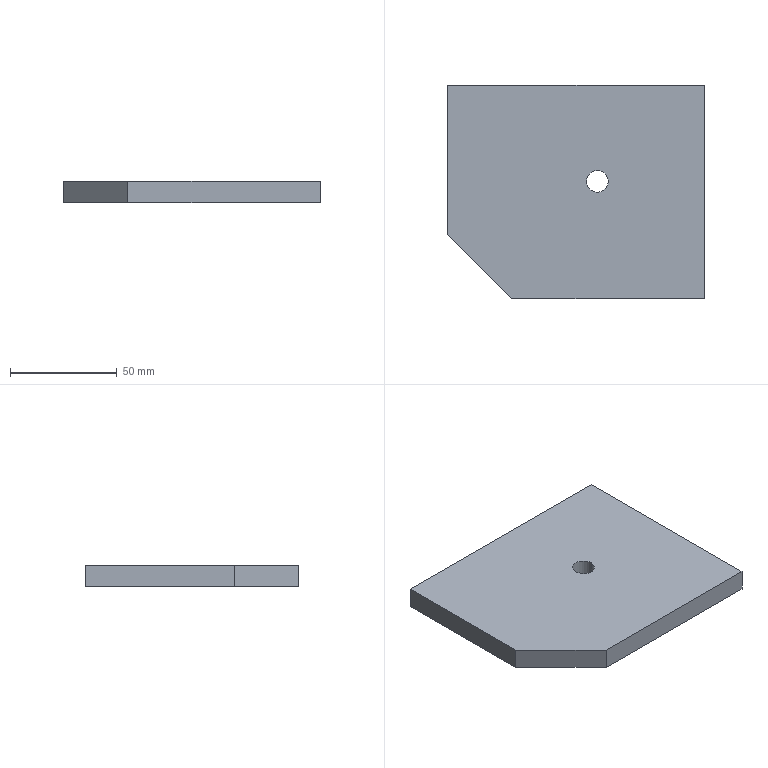Part | SolidWorks | features Extrusion 1, HoleWzd 1 | 1 solid | 9 faces | box 120 x 100 x 10 mm | volume 114683 mm3 | plane 7 | cylinder 2 | commonest cylinder face diameters 10.2 x2
STEP:
#1=CARTESIAN_POINT('',(4.055,5.704,0.));
#2=VERTEX_POINT('',#1);
#3=CARTESIAN_POINT('',(14.255,5.704,0.));
#4=VERTEX_POINT('',#3);
#5=CARTESIAN_POINT('',(9.155,5.704,0.));
#6=DIRECTION('',(0.,0.,1.));
#7=DIRECTION('',(1.,0.,0.));
#8=AXIS2_PLACEMENT_3D('',#5,#6,#7);
#9=CIRCLE('',#8,5.1);
#10=EDGE_CURVE('',#2,#4,#9,.T.);
#11=ORIENTED_EDGE('',*,*,#10,.F.);
#12=CARTESIAN_POINT('',(4.055,5.704,10.));
#13=VERTEX_POINT('',#12);
#14=CARTESIAN_POINT('',(4.055,5.704,10.));
#15=DIRECTION('',(0.,0.,1.));
#16=VECTOR('',#15,1000.);
#17=LINE('',#14,#16);
#18=EDGE_CURVE('',#2,#13,#17,.T.);
#19=ORIENTED_EDGE('',*,*,#18,.T.);
#20=CARTESIAN_POINT('',(14.255,5.704,10.));
#21=VERTEX_POINT('',#20);
#22=CARTESIAN_POINT('',(9.155,5.704,10.));
#23=DIRECTION('',(0.,0.,1.));
#24=DIRECTION('',(1.,0.,0.));
#25=AXIS2_PLACEMENT_3D('',#22,#23,#24);
#26=CIRCLE('',#25,5.1);
#27=EDGE_CURVE('',#13,#21,#26,.T.);
#28=ORIENTED_EDGE('',*,*,#27,.T.);
#29=CARTESIAN_POINT('',(14.255,5.704,10.));
#30=DIRECTION('',(0.,0.,1.));
#31=VECTOR('',#30,1000.);
#32=LINE('',#29,#31);
#33=EDGE_CURVE('',#4,#21,#32,.T.);
#34=ORIENTED_EDGE('',*,*,#33,.F.);
#35=EDGE_LOOP('',(#11,#19,#28,#34));
#36=FACE_OUTER_BOUND('',#35,.T.);
#37=CARTESIAN_POINT('',(9.155,5.704,10.));
#38=DIRECTION('',(0.,0.,1.));
#39=DIRECTION('',(1.,0.,0.));
#40=AXIS2_PLACEMENT_3D('',#37,#38,#39);
#41=CYLINDRICAL_SURFACE('',#40,5.1);
#42=ADVANCED_FACE('',(#36),#41,.F.);
#43=CARTESIAN_POINT('',(59.155,-49.296,0.));
#44=VERTEX_POINT('',#43);
#45=CARTESIAN_POINT('',(59.155,50.704,0.));
#46=VERTEX_POINT('',#45);
#47=CARTESIAN_POINT('',(59.155,50.704,0.));
#48=DIRECTION('',(0.,1.,0.));
#49=VECTOR('',#48,1000.);
#50=LINE('',#47,#49);
#51=EDGE_CURVE('',#44,#46,#50,.T.);
#52=ORIENTED_EDGE('',*,*,#51,.T.);
#53=CARTESIAN_POINT('',(59.155,50.704,10.));
#54=VERTEX_POINT('',#53);
#55=CARTESIAN_POINT('',(59.155,50.704,10.));
#56=DIRECTION('',(0.,0.,-1.));
#57=VECTOR('',#56,1000.);
#58=LINE('',#55,#57);
#59=EDGE_CURVE('',#54,#46,#58,.T.);
#60=ORIENTED_EDGE('',*,*,#59,.F.);
#61=CARTESIAN_POINT('',(59.155,-49.296,10.));
#62=VERTEX_POINT('',#61);
#63=CARTESIAN_POINT('',(59.155,50.704,10.));
#64=DIRECTION('',(0.,1.,0.));
#65=VECTOR('',#64,1000.);
#66=LINE('',#63,#65);
#67=EDGE_CURVE('',#62,#54,#66,.T.);
#68=ORIENTED_EDGE('',*,*,#67,.F.);
#69=CARTESIAN_POINT('',(59.155,-49.296,10.));
#70=DIRECTION('',(0.,0.,-1.));
#71=VECTOR('',#70,1000.);
#72=LINE('',#69,#71);
#73=EDGE_CURVE('',#62,#44,#72,.T.);
#74=ORIENTED_EDGE('',*,*,#73,.T.);
#75=EDGE_LOOP('',(#52,#60,#68,#74));
#76=FACE_OUTER_BOUND('',#75,.T.);
#77=CARTESIAN_POINT('',(59.155,50.704,10.));
#78=DIRECTION('',(-1.,0.,0.));
#79=DIRECTION('',(0.,-1.,0.));
#80=AXIS2_PLACEMENT_3D('',#77,#78,#79);
#81=PLANE('',#80);
#82=ADVANCED_FACE('',(#76),#81,.F.);
#83=CARTESIAN_POINT('',(-60.845,50.704,0.));
#84=VERTEX_POINT('',#83);
#85=CARTESIAN_POINT('',(-60.845,50.704,0.));
#86=DIRECTION('',(-1.,0.,0.));
#87=VECTOR('',#86,1000.);
#88=LINE('',#85,#87);
#89=EDGE_CURVE('',#46,#84,#88,.T.);
#90=ORIENTED_EDGE('',*,*,#89,.T.);
#91=CARTESIAN_POINT('',(-60.845,50.704,10.));
#92=VERTEX_POINT('',#91);
#93=CARTESIAN_POINT('',(-60.845,50.704,10.));
#94=DIRECTION('',(0.,0.,-1.));
#95=VECTOR('',#94,1000.);
#96=LINE('',#93,#95);
#97=EDGE_CURVE('',#92,#84,#96,.T.);
#98=ORIENTED_EDGE('',*,*,#97,.F.);
#99=CARTESIAN_POINT('',(-60.845,50.704,10.));
#100=DIRECTION('',(-1.,0.,0.));
#101=VECTOR('',#100,1000.);
#102=LINE('',#99,#101);
#103=EDGE_CURVE('',#54,#92,#102,.T.);
#104=ORIENTED_EDGE('',*,*,#103,.F.);
#105=ORIENTED_EDGE('',*,*,#59,.T.);
#106=EDGE_LOOP('',(#90,#98,#104,#105));
#107=FACE_OUTER_BOUND('',#106,.T.);
#108=CARTESIAN_POINT('',(-60.845,50.704,10.));
#109=DIRECTION('',(0.,-1.,0.));
#110=DIRECTION('',(0.,0.,-1.));
#111=AXIS2_PLACEMENT_3D('',#108,#109,#110);
#112=PLANE('',#111);
#113=ADVANCED_FACE('',(#107),#112,.F.);
#114=CARTESIAN_POINT('',(-60.845,-19.296,0.));
#115=VERTEX_POINT('',#114);
#116=CARTESIAN_POINT('',(-60.845,50.704,0.));
#117=DIRECTION('',(0.,-1.,0.));
#118=VECTOR('',#117,1000.);
#119=LINE('',#116,#118);
#120=EDGE_CURVE('',#84,#115,#119,.T.);
#121=ORIENTED_EDGE('',*,*,#120,.T.);
#122=CARTESIAN_POINT('',(-60.845,-19.296,10.));
#123=VERTEX_POINT('',#122);
#124=CARTESIAN_POINT('',(-60.845,-19.296,10.));
#125=DIRECTION('',(0.,0.,-1.));
#126=VECTOR('',#125,1000.);
#127=LINE('',#124,#126);
#128=EDGE_CURVE('',#123,#115,#127,.T.);
#129=ORIENTED_EDGE('',*,*,#128,.F.);
#130=CARTESIAN_POINT('',(-60.845,50.704,10.));
#131=DIRECTION('',(0.,-1.,0.));
#132=VECTOR('',#131,1000.);
#133=LINE('',#130,#132);
#134=EDGE_CURVE('',#92,#123,#133,.T.);
#135=ORIENTED_EDGE('',*,*,#134,.F.);
#136=ORIENTED_EDGE('',*,*,#97,.T.);
#137=EDGE_LOOP('',(#121,#129,#135,#136));
#138=FACE_OUTER_BOUND('',#137,.T.);
#139=CARTESIAN_POINT('',(-60.845,50.704,10.));
#140=DIRECTION('',(1.,0.,0.));
#141=DIRECTION('',(0.,0.,-1.));
#142=AXIS2_PLACEMENT_3D('',#139,#140,#141);
#143=PLANE('',#142);
#144=ADVANCED_FACE('',(#138),#143,.F.);
#145=CARTESIAN_POINT('',(-30.845,-49.296,0.));
#146=VERTEX_POINT('',#145);
#147=CARTESIAN_POINT('',(-30.845,-49.296,0.));
#148=DIRECTION('',(0.7071,-0.7071,0.));
#149=VECTOR('',#148,1000.);
#150=LINE('',#147,#149);
#151=EDGE_CURVE('',#115,#146,#150,.T.);
#152=ORIENTED_EDGE('',*,*,#151,.T.);
#153=CARTESIAN_POINT('',(-30.845,-49.296,10.));
#154=VERTEX_POINT('',#153);
#155=CARTESIAN_POINT('',(-30.845,-49.296,10.));
#156=DIRECTION('',(0.,0.,-1.));
#157=VECTOR('',#156,1000.);
#158=LINE('',#155,#157);
#159=EDGE_CURVE('',#154,#146,#158,.T.);
#160=ORIENTED_EDGE('',*,*,#159,.F.);
#161=CARTESIAN_POINT('',(-30.845,-49.296,10.));
#162=DIRECTION('',(0.7071,-0.7071,0.));
#163=VECTOR('',#162,1000.);
#164=LINE('',#161,#163);
#165=EDGE_CURVE('',#123,#154,#164,.T.);
#166=ORIENTED_EDGE('',*,*,#165,.F.);
#167=ORIENTED_EDGE('',*,*,#128,.T.);
#168=EDGE_LOOP('',(#152,#160,#166,#167));
#169=FACE_OUTER_BOUND('',#168,.T.);
#170=CARTESIAN_POINT('',(-30.845,-49.296,10.));
#171=DIRECTION('',(0.7071,0.7071,0.));
#172=DIRECTION('',(-0.7071,0.7071,0.));
#173=AXIS2_PLACEMENT_3D('',#170,#171,#172);
#174=PLANE('',#173);
#175=ADVANCED_FACE('',(#169),#174,.F.);
#176=CARTESIAN_POINT('',(-30.845,-49.296,0.));
#177=DIRECTION('',(1.,0.,0.));
#178=VECTOR('',#177,1000.);
#179=LINE('',#176,#178);
#180=EDGE_CURVE('',#146,#44,#179,.T.);
#181=ORIENTED_EDGE('',*,*,#180,.T.);
#182=ORIENTED_EDGE('',*,*,#73,.F.);
#183=CARTESIAN_POINT('',(-30.845,-49.296,10.));
#184=DIRECTION('',(1.,0.,0.));
#185=VECTOR('',#184,1000.);
#186=LINE('',#183,#185);
#187=EDGE_CURVE('',#154,#62,#186,.T.);
#188=ORIENTED_EDGE('',*,*,#187,.F.);
#189=ORIENTED_EDGE('',*,*,#159,.T.);
#190=EDGE_LOOP('',(#181,#182,#188,#189));
#191=FACE_OUTER_BOUND('',#190,.T.);
#192=CARTESIAN_POINT('',(-30.845,-49.296,10.));
#193=DIRECTION('',(0.,1.,0.));
#194=DIRECTION('',(0.,0.,1.));
#195=AXIS2_PLACEMENT_3D('',#192,#193,#194);
#196=PLANE('',#195);
#197=ADVANCED_FACE('',(#191),#196,.F.);
#198=CARTESIAN_POINT('',(9.155,5.704,10.));
#199=DIRECTION('',(0.,0.,1.));
#200=DIRECTION('',(1.,0.,0.));
#201=AXIS2_PLACEMENT_3D('',#198,#199,#200);
#202=CIRCLE('',#201,5.1);
#203=EDGE_CURVE('',#21,#13,#202,.T.);
#204=ORIENTED_EDGE('',*,*,#203,.F.);
#205=ORIENTED_EDGE('',*,*,#27,.F.);
#206=EDGE_LOOP('',(#204,#205));
#207=FACE_BOUND('',#206,.T.);
#208=ORIENTED_EDGE('',*,*,#67,.T.);
#209=ORIENTED_EDGE('',*,*,#103,.T.);
#210=ORIENTED_EDGE('',*,*,#134,.T.);
#211=ORIENTED_EDGE('',*,*,#165,.T.);
#212=ORIENTED_EDGE('',*,*,#187,.T.);
#213=EDGE_LOOP('',(#208,#209,#210,#211,#212));
#214=FACE_OUTER_BOUND('',#213,.T.);
#215=CARTESIAN_POINT('',(0.,0.,10.));
#216=DIRECTION('',(0.,0.,1.));
#217=DIRECTION('',(1.,0.,0.));
#218=AXIS2_PLACEMENT_3D('',#215,#216,#217);
#219=PLANE('',#218);
#220=ADVANCED_FACE('',(#207,#214),#219,.T.);
#221=CARTESIAN_POINT('',(9.155,5.704,0.));
#222=DIRECTION('',(0.,0.,1.));
#223=DIRECTION('',(1.,0.,0.));
#224=AXIS2_PLACEMENT_3D('',#221,#222,#223);
#225=CIRCLE('',#224,5.1);
#226=EDGE_CURVE('',#4,#2,#225,.T.);
#227=ORIENTED_EDGE('',*,*,#226,.T.);
#228=ORIENTED_EDGE('',*,*,#10,.T.);
#229=EDGE_LOOP('',(#227,#228));
#230=FACE_BOUND('',#229,.T.);
#231=ORIENTED_EDGE('',*,*,#51,.F.);
#232=ORIENTED_EDGE('',*,*,#180,.F.);
#233=ORIENTED_EDGE('',*,*,#151,.F.);
#234=ORIENTED_EDGE('',*,*,#120,.F.);
#235=ORIENTED_EDGE('',*,*,#89,.F.);
#236=EDGE_LOOP('',(#231,#232,#233,#234,#235));
#237=FACE_OUTER_BOUND('',#236,.T.);
#238=CARTESIAN_POINT('',(0.,0.,0.));
#239=DIRECTION('',(0.,0.,1.));
#240=DIRECTION('',(1.,0.,0.));
#241=AXIS2_PLACEMENT_3D('',#238,#239,#240);
#242=PLANE('',#241);
#243=ADVANCED_FACE('',(#230,#237),#242,.F.);
#244=ORIENTED_EDGE('',*,*,#18,.F.);
#245=ORIENTED_EDGE('',*,*,#226,.F.);
#246=ORIENTED_EDGE('',*,*,#33,.T.);
#247=ORIENTED_EDGE('',*,*,#203,.T.);
#248=EDGE_LOOP('',(#244,#245,#246,#247));
#249=FACE_OUTER_BOUND('',#248,.T.);
#250=CARTESIAN_POINT('',(9.155,5.704,10.));
#251=DIRECTION('',(0.,0.,1.));
#252=DIRECTION('',(1.,0.,0.));
#253=AXIS2_PLACEMENT_3D('',#250,#251,#252);
#254=CYLINDRICAL_SURFACE('',#253,5.1);
#255=ADVANCED_FACE('',(#249),#254,.F.);
#256=CLOSED_SHELL('',(#42,#82,#113,#144,#175,#197,#220,#243,#255));
#257=MANIFOLD_SOLID_BREP('',#256);
#258=CARTESIAN_POINT('',(0.,0.,0.));
#259=DIRECTION('',(0.,0.,1.));
#260=DIRECTION('',(1.,0.,0.));
#261=AXIS2_PLACEMENT_3D('',#258,#259,#260);
#262=(LENGTH_UNIT()NAMED_UNIT(*)SI_UNIT(.MILLI.,.METRE.));
#263=UNCERTAINTY_MEASURE_WITH_UNIT(LENGTH_MEASURE(0.00001),#262,'','');
#264=(NAMED_UNIT(*)PLANE_ANGLE_UNIT()SI_UNIT($,.RADIAN.));
#265=(NAMED_UNIT(*)SI_UNIT($,.STERADIAN.)SOLID_ANGLE_UNIT());
#266=(GEOMETRIC_REPRESENTATION_CONTEXT(3)GLOBAL_UNCERTAINTY_ASSIGNED_CONTEXT((#263))GLOBAL_UNIT_ASSIGNED_CONTEXT((#262,#264,#265))REPRESENTATION_CONTEXT('',''));
#267=ADVANCED_BREP_SHAPE_REPRESENTATION('',(#257,#261),#266);